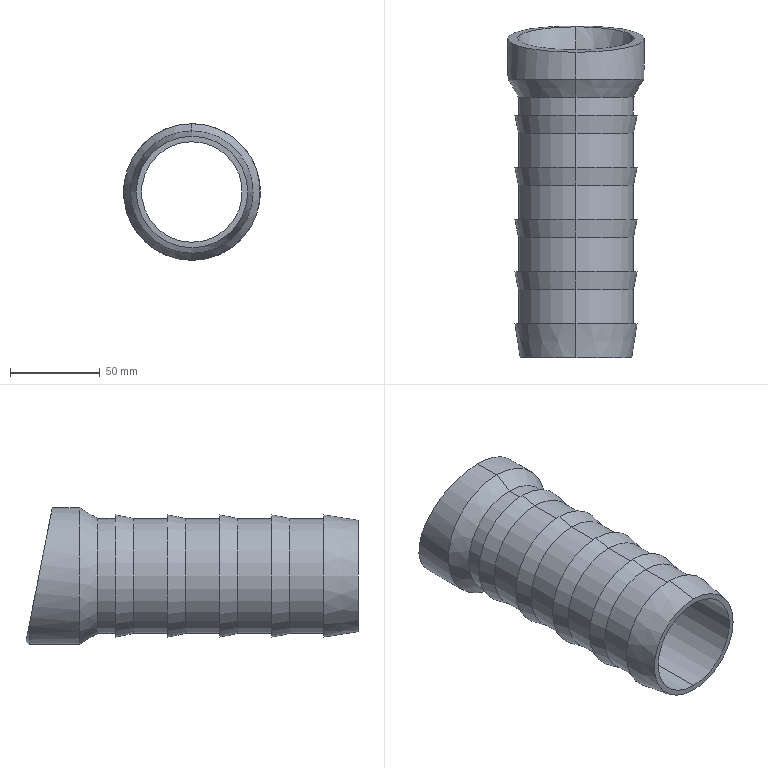Part | SolidWorks | features ICE 2, BlendCut 1, Revolution 1 | 1 solid | 37 faces | box 76 x 184.67 x 76 mm | volume 170240 mm3 | cone 16 | cylinder 14 | plane 7 | commonest cylinder face diameters 64 x10 56 x2 76 x2
STEP:
#1=CARTESIAN_POINT('',(0.,62.5,-28.));
#2=VERTEX_POINT('',#1);
#3=CARTESIAN_POINT('',(0.,62.5,28.));
#4=VERTEX_POINT('',#3);
#5=CARTESIAN_POINT('',(0.,62.5,0.));
#6=DIRECTION('',(0.,1.,0.));
#7=DIRECTION('',(0.,0.,1.));
#8=AXIS2_PLACEMENT_3D('',#5,#6,#7);
#9=CIRCLE('',#8,28.);
#10=EDGE_CURVE('',#2,#4,#9,.T.);
#11=ORIENTED_EDGE('',*,*,#10,.F.);
#12=CARTESIAN_POINT('',(0.,91.678,-33.836));
#13=VERTEX_POINT('',#12);
#14=CARTESIAN_POINT('',(0.,62.5,-28.));
#15=DIRECTION('',(0.,0.9806,-0.1961));
#16=VECTOR('',#15,1000.);
#17=LINE('',#14,#16);
#18=EDGE_CURVE('',#2,#13,#17,.T.);
#19=ORIENTED_EDGE('',*,*,#18,.T.);
#20=CARTESIAN_POINT('',(0.,78.829,31.266));
#21=VERTEX_POINT('',#20);
#22=CARTESIAN_POINT('',(0.,91.678,-33.836));
#23=CARTESIAN_POINT('',(-65.051,91.678,-33.836));
#24=CARTESIAN_POINT('',(-65.051,78.829,31.266));
#25=CARTESIAN_POINT('',(0.,78.829,31.266));
#26=(BOUNDED_CURVE()B_SPLINE_CURVE(3,(#22,#23,#24,#25),.UNSPECIFIED.,.F.,.F.)B_SPLINE_CURVE_WITH_KNOTS((4,4),(0.,3.142),.UNSPECIFIED.)CURVE()GEOMETRIC_REPRESENTATION_ITEM()RATIONAL_B_SPLINE_CURVE((1.,0.3333,0.3333,1.))REPRESENTATION_ITEM(''));
#27=EDGE_CURVE('',#13,#21,#26,.T.);
#28=ORIENTED_EDGE('',*,*,#27,.T.);
#29=CARTESIAN_POINT('',(0.,62.5,28.));
#30=DIRECTION('',(0.,0.9806,0.1961));
#31=VECTOR('',#30,1000.);
#32=LINE('',#29,#31);
#33=EDGE_CURVE('',#4,#21,#32,.T.);
#34=ORIENTED_EDGE('',*,*,#33,.F.);
#35=EDGE_LOOP('',(#11,#19,#28,#34));
#36=FACE_OUTER_BOUND('',#35,.T.);
#37=CARTESIAN_POINT('',(0.,62.5,0.));
#38=DIRECTION('',(0.,1.,0.));
#39=DIRECTION('',(0.,0.,1.));
#40=AXIS2_PLACEMENT_3D('',#37,#38,#39);
#41=CONICAL_SURFACE('',#40,28.,0.1974);
#42=ADVANCED_FACE('',(#36),#41,.F.);
#43=CARTESIAN_POINT('',(0.,-92.5,28.));
#44=VERTEX_POINT('',#43);
#45=CARTESIAN_POINT('',(0.,-92.5,-28.));
#46=VERTEX_POINT('',#45);
#47=CARTESIAN_POINT('',(0.,-92.5,0.));
#48=DIRECTION('',(0.,-1.,0.));
#49=DIRECTION('',(0.,0.,1.));
#50=AXIS2_PLACEMENT_3D('',#47,#48,#49);
#51=CIRCLE('',#50,28.);
#52=EDGE_CURVE('',#44,#46,#51,.T.);
#53=ORIENTED_EDGE('',*,*,#52,.T.);
#54=CARTESIAN_POINT('',(0.,-171.696,-28.));
#55=DIRECTION('',(0.,1.,0.));
#56=VECTOR('',#55,1000.);
#57=LINE('',#54,#56);
#58=EDGE_CURVE('',#46,#2,#57,.T.);
#59=ORIENTED_EDGE('',*,*,#58,.T.);
#60=ORIENTED_EDGE('',*,*,#10,.T.);
#61=CARTESIAN_POINT('',(0.,-171.696,28.));
#62=DIRECTION('',(0.,1.,0.));
#63=VECTOR('',#62,1000.);
#64=LINE('',#61,#63);
#65=EDGE_CURVE('',#44,#4,#64,.T.);
#66=ORIENTED_EDGE('',*,*,#65,.F.);
#67=EDGE_LOOP('',(#53,#59,#60,#66));
#68=FACE_OUTER_BOUND('',#67,.T.);
#69=CARTESIAN_POINT('',(0.,-171.696,0.));
#70=DIRECTION('',(0.,1.,0.));
#71=DIRECTION('',(0.,0.,1.));
#72=AXIS2_PLACEMENT_3D('',#69,#70,#71);
#73=CYLINDRICAL_SURFACE('',#72,28.);
#74=ADVANCED_FACE('',(#68),#73,.F.);
#75=CARTESIAN_POINT('',(0.,-54.5,32.));
#76=VERTEX_POINT('',#75);
#77=CARTESIAN_POINT('',(0.,-54.5,-32.));
#78=VERTEX_POINT('',#77);
#79=CARTESIAN_POINT('',(0.,-54.5,0.));
#80=DIRECTION('',(0.,1.,0.));
#81=DIRECTION('',(0.,0.,1.));
#82=AXIS2_PLACEMENT_3D('',#79,#80,#81);
#83=CIRCLE('',#82,32.);
#84=EDGE_CURVE('',#76,#78,#83,.T.);
#85=ORIENTED_EDGE('',*,*,#84,.T.);
#86=CARTESIAN_POINT('',(0.,-44.5,-34.));
#87=VERTEX_POINT('',#86);
#88=CARTESIAN_POINT('',(0.,-54.5,-32.));
#89=DIRECTION('',(0.,0.9806,-0.1961));
#90=VECTOR('',#89,1000.);
#91=LINE('',#88,#90);
#92=EDGE_CURVE('',#78,#87,#91,.T.);
#93=ORIENTED_EDGE('',*,*,#92,.T.);
#94=CARTESIAN_POINT('',(0.,-44.5,34.));
#95=VERTEX_POINT('',#94);
#96=CARTESIAN_POINT('',(0.,-44.5,0.));
#97=DIRECTION('',(0.,1.,0.));
#98=DIRECTION('',(0.,0.,1.));
#99=AXIS2_PLACEMENT_3D('',#96,#97,#98);
#100=CIRCLE('',#99,34.);
#101=EDGE_CURVE('',#95,#87,#100,.T.);
#102=ORIENTED_EDGE('',*,*,#101,.F.);
#103=CARTESIAN_POINT('',(0.,-54.5,32.));
#104=DIRECTION('',(0.,0.9806,0.1961));
#105=VECTOR('',#104,1000.);
#106=LINE('',#103,#105);
#107=EDGE_CURVE('',#76,#95,#106,.T.);
#108=ORIENTED_EDGE('',*,*,#107,.F.);
#109=EDGE_LOOP('',(#85,#93,#102,#108));
#110=FACE_OUTER_BOUND('',#109,.T.);
#111=CARTESIAN_POINT('',(0.,-54.5,0.));
#112=DIRECTION('',(0.,1.,0.));
#113=DIRECTION('',(0.,0.,1.));
#114=AXIS2_PLACEMENT_3D('',#111,#112,#113);
#115=CONICAL_SURFACE('',#114,32.,0.1974);
#116=ADVANCED_FACE('',(#110),#115,.T.);
#117=CARTESIAN_POINT('',(0.,-73.5,32.));
#118=VERTEX_POINT('',#117);
#119=CARTESIAN_POINT('',(0.,-73.5,-32.));
#120=VERTEX_POINT('',#119);
#121=CARTESIAN_POINT('',(0.,-73.5,0.));
#122=DIRECTION('',(0.,1.,0.));
#123=DIRECTION('',(0.,0.,1.));
#124=AXIS2_PLACEMENT_3D('',#121,#122,#123);
#125=CIRCLE('',#124,32.);
#126=EDGE_CURVE('',#118,#120,#125,.T.);
#127=ORIENTED_EDGE('',*,*,#126,.T.);
#128=CARTESIAN_POINT('',(0.,92.5,-32.));
#129=DIRECTION('',(0.,1.,0.));
#130=VECTOR('',#129,1000.);
#131=LINE('',#128,#130);
#132=EDGE_CURVE('',#120,#78,#131,.T.);
#133=ORIENTED_EDGE('',*,*,#132,.T.);
#134=ORIENTED_EDGE('',*,*,#84,.F.);
#135=CARTESIAN_POINT('',(0.,92.5,32.));
#136=DIRECTION('',(0.,1.,0.));
#137=VECTOR('',#136,1000.);
#138=LINE('',#135,#137);
#139=EDGE_CURVE('',#118,#76,#138,.T.);
#140=ORIENTED_EDGE('',*,*,#139,.F.);
#141=EDGE_LOOP('',(#127,#133,#134,#140));
#142=FACE_OUTER_BOUND('',#141,.T.);
#143=CARTESIAN_POINT('',(0.,92.5,0.));
#144=DIRECTION('',(0.,1.,0.));
#145=DIRECTION('',(0.,0.,1.));
#146=AXIS2_PLACEMENT_3D('',#143,#144,#145);
#147=CYLINDRICAL_SURFACE('',#146,32.);
#148=ADVANCED_FACE('',(#142),#147,.T.);
#149=CARTESIAN_POINT('',(0.,-92.5,31.));
#150=VERTEX_POINT('',#149);
#151=CARTESIAN_POINT('',(0.,-92.5,-31.));
#152=VERTEX_POINT('',#151);
#153=CARTESIAN_POINT('',(0.,-92.5,0.));
#154=DIRECTION('',(0.,1.,0.));
#155=DIRECTION('',(0.,0.,1.));
#156=AXIS2_PLACEMENT_3D('',#153,#154,#155);
#157=CIRCLE('',#156,31.);
#158=EDGE_CURVE('',#150,#152,#157,.T.);
#159=ORIENTED_EDGE('',*,*,#158,.T.);
#160=CARTESIAN_POINT('',(0.,-73.5,-34.));
#161=VERTEX_POINT('',#160);
#162=CARTESIAN_POINT('',(0.,-92.5,-31.));
#163=DIRECTION('',(0.,0.9878,-0.156));
#164=VECTOR('',#163,1000.);
#165=LINE('',#162,#164);
#166=EDGE_CURVE('',#152,#161,#165,.T.);
#167=ORIENTED_EDGE('',*,*,#166,.T.);
#168=CARTESIAN_POINT('',(0.,-73.5,34.));
#169=VERTEX_POINT('',#168);
#170=CARTESIAN_POINT('',(0.,-73.5,0.));
#171=DIRECTION('',(0.,1.,0.));
#172=DIRECTION('',(0.,0.,1.));
#173=AXIS2_PLACEMENT_3D('',#170,#171,#172);
#174=CIRCLE('',#173,34.);
#175=EDGE_CURVE('',#169,#161,#174,.T.);
#176=ORIENTED_EDGE('',*,*,#175,.F.);
#177=CARTESIAN_POINT('',(0.,-92.5,31.));
#178=DIRECTION('',(0.,0.9878,0.156));
#179=VECTOR('',#178,1000.);
#180=LINE('',#177,#179);
#181=EDGE_CURVE('',#150,#169,#180,.T.);
#182=ORIENTED_EDGE('',*,*,#181,.F.);
#183=EDGE_LOOP('',(#159,#167,#176,#182));
#184=FACE_OUTER_BOUND('',#183,.T.);
#185=CARTESIAN_POINT('',(0.,-92.5,0.));
#186=DIRECTION('',(0.,1.,0.));
#187=DIRECTION('',(0.,0.,1.));
#188=AXIS2_PLACEMENT_3D('',#185,#186,#187);
#189=CONICAL_SURFACE('',#188,31.,0.1566);
#190=ADVANCED_FACE('',(#184),#189,.T.);
#191=CARTESIAN_POINT('',(-25.835,90.5,-27.867));
#192=VERTEX_POINT('',#191);
#193=CARTESIAN_POINT('',(0.,92.17,-36.33));
#194=VERTEX_POINT('',#193);
#195=CARTESIAN_POINT('',(-25.835,90.5,-27.867));
#196=CARTESIAN_POINT('',(-18.239,91.595,-33.416));
#197=CARTESIAN_POINT('',(-9.343,92.17,-36.33));
#198=CARTESIAN_POINT('',(0.,92.17,-36.33));
#199=(BOUNDED_CURVE()B_SPLINE_CURVE(3,(#195,#196,#197,#198),.UNSPECIFIED.,.F.,.F.)B_SPLINE_CURVE_WITH_KNOTS((4,4),(2.52,3.142),.UNSPECIFIED.)CURVE()GEOMETRIC_REPRESENTATION_ITEM()RATIONAL_B_SPLINE_CURVE((1.,0.9681,0.9681,1.))REPRESENTATION_ITEM(''));
#200=EDGE_CURVE('',#192,#194,#199,.T.);
#201=ORIENTED_EDGE('',*,*,#200,.T.);
#202=CARTESIAN_POINT('',(0.,90.5,-38.));
#203=VERTEX_POINT('',#202);
#204=CARTESIAN_POINT('',(0.,90.5,-38.));
#205=DIRECTION('',(0.,-0.7071,-0.7071));
#206=VECTOR('',#205,1000.);
#207=LINE('',#204,#206);
#208=EDGE_CURVE('',#194,#203,#207,.T.);
#209=ORIENTED_EDGE('',*,*,#208,.T.);
#210=CARTESIAN_POINT('',(0.,90.5,0.));
#211=DIRECTION('',(0.,1.,0.));
#212=DIRECTION('',(0.,0.,1.));
#213=AXIS2_PLACEMENT_3D('',#210,#211,#212);
#214=CIRCLE('',#213,38.);
#215=EDGE_CURVE('',#203,#192,#214,.T.);
#216=ORIENTED_EDGE('',*,*,#215,.T.);
#217=EDGE_LOOP('',(#201,#209,#216));
#218=FACE_OUTER_BOUND('',#217,.T.);
#219=CARTESIAN_POINT('',(0.,90.5,0.));
#220=DIRECTION('',(0.,-1.,0.));
#221=DIRECTION('',(0.,0.,-1.));
#222=AXIS2_PLACEMENT_3D('',#219,#220,#221);
#223=CONICAL_SURFACE('',#222,38.,0.7854);
#224=ADVANCED_FACE('',(#218),#223,.T.);
#225=CARTESIAN_POINT('',(0.,62.5,38.));
#226=VERTEX_POINT('',#225);
#227=CARTESIAN_POINT('',(0.,62.5,-38.));
#228=VERTEX_POINT('',#227);
#229=CARTESIAN_POINT('',(0.,62.5,0.));
#230=DIRECTION('',(0.,1.,0.));
#231=DIRECTION('',(0.,0.,1.));
#232=AXIS2_PLACEMENT_3D('',#229,#230,#231);
#233=CIRCLE('',#232,38.);
#234=EDGE_CURVE('',#226,#228,#233,.T.);
#235=ORIENTED_EDGE('',*,*,#234,.T.);
#236=CARTESIAN_POINT('',(0.,92.5,-38.));
#237=DIRECTION('',(0.,1.,0.));
#238=VECTOR('',#237,1000.);
#239=LINE('',#236,#238);
#240=EDGE_CURVE('',#228,#203,#239,.T.);
#241=ORIENTED_EDGE('',*,*,#240,.T.);
#242=CARTESIAN_POINT('',(25.835,90.5,-27.867));
#243=VERTEX_POINT('',#242);
#244=CARTESIAN_POINT('',(0.,90.5,0.));
#245=DIRECTION('',(0.,1.,0.));
#246=DIRECTION('',(0.,0.,1.));
#247=AXIS2_PLACEMENT_3D('',#244,#245,#246);
#248=CIRCLE('',#247,38.);
#249=EDGE_CURVE('',#243,#203,#248,.T.);
#250=ORIENTED_EDGE('',*,*,#249,.F.);
#251=CARTESIAN_POINT('',(0.,77.5,38.));
#252=VERTEX_POINT('',#251);
#253=CARTESIAN_POINT('',(25.835,90.5,-27.867));
#254=CARTESIAN_POINT('',(55.821,85.013,-0.06669));
#255=CARTESIAN_POINT('',(40.89,77.5,38.));
#256=CARTESIAN_POINT('',(0.,77.5,38.));
#257=(BOUNDED_CURVE()B_SPLINE_CURVE(3,(#253,#254,#255,#256),.UNSPECIFIED.,.F.,.F.)B_SPLINE_CURVE_WITH_KNOTS((4,4),(0.7476,3.142),.UNSPECIFIED.)CURVE()GEOMETRIC_REPRESENTATION_ITEM()RATIONAL_B_SPLINE_CURVE((1.,0.5768,0.5768,1.))REPRESENTATION_ITEM(''));
#258=EDGE_CURVE('',#243,#252,#257,.T.);
#259=ORIENTED_EDGE('',*,*,#258,.T.);
#260=CARTESIAN_POINT('',(0.,92.5,38.));
#261=DIRECTION('',(0.,1.,0.));
#262=VECTOR('',#261,1000.);
#263=LINE('',#260,#262);
#264=EDGE_CURVE('',#226,#252,#263,.T.);
#265=ORIENTED_EDGE('',*,*,#264,.F.);
#266=EDGE_LOOP('',(#235,#241,#250,#259,#265));
#267=FACE_OUTER_BOUND('',#266,.T.);
#268=CARTESIAN_POINT('',(0.,92.5,0.));
#269=DIRECTION('',(0.,1.,0.));
#270=DIRECTION('',(0.,0.,1.));
#271=AXIS2_PLACEMENT_3D('',#268,#269,#270);
#272=CYLINDRICAL_SURFACE('',#271,38.);
#273=ADVANCED_FACE('',(#267),#272,.T.);
#274=CARTESIAN_POINT('',(0.,52.5,32.));
#275=VERTEX_POINT('',#274);
#276=CARTESIAN_POINT('',(0.,52.5,-32.));
#277=VERTEX_POINT('',#276);
#278=CARTESIAN_POINT('',(0.,52.5,0.));
#279=DIRECTION('',(0.,1.,0.));
#280=DIRECTION('',(0.,0.,1.));
#281=AXIS2_PLACEMENT_3D('',#278,#279,#280);
#282=CIRCLE('',#281,32.);
#283=EDGE_CURVE('',#275,#277,#282,.T.);
#284=ORIENTED_EDGE('',*,*,#283,.T.);
#285=CARTESIAN_POINT('',(0.,52.5,-32.));
#286=DIRECTION('',(0.,0.8575,-0.5145));
#287=VECTOR('',#286,1000.);
#288=LINE('',#285,#287);
#289=EDGE_CURVE('',#277,#228,#288,.T.);
#290=ORIENTED_EDGE('',*,*,#289,.T.);
#291=ORIENTED_EDGE('',*,*,#234,.F.);
#292=CARTESIAN_POINT('',(0.,52.5,32.));
#293=DIRECTION('',(0.,0.8575,0.5145));
#294=VECTOR('',#293,1000.);
#295=LINE('',#292,#294);
#296=EDGE_CURVE('',#275,#226,#295,.T.);
#297=ORIENTED_EDGE('',*,*,#296,.F.);
#298=EDGE_LOOP('',(#284,#290,#291,#297));
#299=FACE_OUTER_BOUND('',#298,.T.);
#300=CARTESIAN_POINT('',(0.,52.5,0.));
#301=DIRECTION('',(0.,1.,0.));
#302=DIRECTION('',(0.,0.,1.));
#303=AXIS2_PLACEMENT_3D('',#300,#301,#302);
#304=CONICAL_SURFACE('',#303,32.,0.5404);
#305=ADVANCED_FACE('',(#299),#304,.T.);
#306=CARTESIAN_POINT('',(0.,42.5,32.));
#307=VERTEX_POINT('',#306);
#308=CARTESIAN_POINT('',(0.,42.5,-32.));
#309=VERTEX_POINT('',#308);
#310=CARTESIAN_POINT('',(0.,42.5,0.));
#311=DIRECTION('',(0.,1.,0.));
#312=DIRECTION('',(0.,0.,1.));
#313=AXIS2_PLACEMENT_3D('',#310,#311,#312);
#314=CIRCLE('',#313,32.);
#315=EDGE_CURVE('',#307,#309,#314,.T.);
#316=ORIENTED_EDGE('',*,*,#315,.T.);
#317=CARTESIAN_POINT('',(0.,92.5,-32.));
#318=DIRECTION('',(0.,1.,0.));
#319=VECTOR('',#318,1000.);
#320=LINE('',#317,#319);
#321=EDGE_CURVE('',#309,#277,#320,.T.);
#322=ORIENTED_EDGE('',*,*,#321,.T.);
#323=ORIENTED_EDGE('',*,*,#283,.F.);
#324=CARTESIAN_POINT('',(0.,92.5,32.));
#325=DIRECTION('',(0.,1.,0.));
#326=VECTOR('',#325,1000.);
#327=LINE('',#324,#326);
#328=EDGE_CURVE('',#307,#275,#327,.T.);
#329=ORIENTED_EDGE('',*,*,#328,.F.);
#330=EDGE_LOOP('',(#316,#322,#323,#329));
#331=FACE_OUTER_BOUND('',#330,.T.);
#332=CARTESIAN_POINT('',(0.,92.5,0.));
#333=DIRECTION('',(0.,1.,0.));
#334=DIRECTION('',(0.,0.,1.));
#335=AXIS2_PLACEMENT_3D('',#332,#333,#334);
#336=CYLINDRICAL_SURFACE('',#335,32.);
#337=ADVANCED_FACE('',(#331),#336,.T.);
#338=CARTESIAN_POINT('',(0.,32.5,32.));
#339=VERTEX_POINT('',#338);
#340=CARTESIAN_POINT('',(0.,32.5,-32.));
#341=VERTEX_POINT('',#340);
#342=CARTESIAN_POINT('',(0.,32.5,0.));
#343=DIRECTION('',(0.,1.,0.));
#344=DIRECTION('',(0.,0.,1.));
#345=AXIS2_PLACEMENT_3D('',#342,#343,#344);
#346=CIRCLE('',#345,32.);
#347=EDGE_CURVE('',#339,#341,#346,.T.);
#348=ORIENTED_EDGE('',*,*,#347,.T.);
#349=CARTESIAN_POINT('',(0.,42.5,-34.));
#350=VERTEX_POINT('',#349);
#351=CARTESIAN_POINT('',(0.,32.5,-32.));
#352=DIRECTION('',(0.,0.9806,-0.1961));
#353=VECTOR('',#352,1000.);
#354=LINE('',#351,#353);
#355=EDGE_CURVE('',#341,#350,#354,.T.);
#356=ORIENTED_EDGE('',*,*,#355,.T.);
#357=CARTESIAN_POINT('',(0.,42.5,34.));
#358=VERTEX_POINT('',#357);
#359=CARTESIAN_POINT('',(0.,42.5,0.));
#360=DIRECTION('',(0.,1.,0.));
#361=DIRECTION('',(0.,0.,1.));
#362=AXIS2_PLACEMENT_3D('',#359,#360,#361);
#363=CIRCLE('',#362,34.);
#364=EDGE_CURVE('',#358,#350,#363,.T.);
#365=ORIENTED_EDGE('',*,*,#364,.F.);
#366=CARTESIAN_POINT('',(0.,32.5,32.));
#367=DIRECTION('',(0.,0.9806,0.1961));
#368=VECTOR('',#367,1000.);
#369=LINE('',#366,#368);
#370=EDGE_CURVE('',#339,#358,#369,.T.);
#371=ORIENTED_EDGE('',*,*,#370,.F.);
#372=EDGE_LOOP('',(#348,#356,#365,#371));
#373=FACE_OUTER_BOUND('',#372,.T.);
#374=CARTESIAN_POINT('',(0.,32.5,0.));
#375=DIRECTION('',(0.,1.,0.));
#376=DIRECTION('',(0.,0.,1.));
#377=AXIS2_PLACEMENT_3D('',#374,#375,#376);
#378=CONICAL_SURFACE('',#377,32.,0.1974);
#379=ADVANCED_FACE('',(#373),#378,.T.);
#380=CARTESIAN_POINT('',(0.,13.5,32.));
#381=VERTEX_POINT('',#380);
#382=CARTESIAN_POINT('',(0.,13.5,-32.));
#383=VERTEX_POINT('',#382);
#384=CARTESIAN_POINT('',(0.,13.5,0.));
#385=DIRECTION('',(0.,1.,0.));
#386=DIRECTION('',(0.,0.,1.));
#387=AXIS2_PLACEMENT_3D('',#384,#385,#386);
#388=CIRCLE('',#387,32.);
#389=EDGE_CURVE('',#381,#383,#388,.T.);
#390=ORIENTED_EDGE('',*,*,#389,.T.);
#391=CARTESIAN_POINT('',(0.,92.5,-32.));
#392=DIRECTION('',(0.,1.,0.));
#393=VECTOR('',#392,1000.);
#394=LINE('',#391,#393);
#395=EDGE_CURVE('',#383,#341,#394,.T.);
#396=ORIENTED_EDGE('',*,*,#395,.T.);
#397=ORIENTED_EDGE('',*,*,#347,.F.);
#398=CARTESIAN_POINT('',(0.,92.5,32.));
#399=DIRECTION('',(0.,1.,0.));
#400=VECTOR('',#399,1000.);
#401=LINE('',#398,#400);
#402=EDGE_CURVE('',#381,#339,#401,.T.);
#403=ORIENTED_EDGE('',*,*,#402,.F.);
#404=EDGE_LOOP('',(#390,#396,#397,#403));
#405=FACE_OUTER_BOUND('',#404,.T.);
#406=CARTESIAN_POINT('',(0.,92.5,0.));
#407=DIRECTION('',(0.,1.,0.));
#408=DIRECTION('',(0.,0.,1.));
#409=AXIS2_PLACEMENT_3D('',#406,#407,#408);
#410=CYLINDRICAL_SURFACE('',#409,32.);
#411=ADVANCED_FACE('',(#405),#410,.T.);
#412=CARTESIAN_POINT('',(0.,3.5,32.));
#413=VERTEX_POINT('',#412);
#414=CARTESIAN_POINT('',(0.,3.5,-32.));
#415=VERTEX_POINT('',#414);
#416=CARTESIAN_POINT('',(0.,3.5,0.));
#417=DIRECTION('',(0.,1.,0.));
#418=DIRECTION('',(0.,0.,1.));
#419=AXIS2_PLACEMENT_3D('',#416,#417,#418);
#420=CIRCLE('',#419,32.);
#421=EDGE_CURVE('',#413,#415,#420,.T.);
#422=ORIENTED_EDGE('',*,*,#421,.T.);
#423=CARTESIAN_POINT('',(0.,13.5,-34.));
#424=VERTEX_POINT('',#423);
#425=CARTESIAN_POINT('',(0.,3.5,-32.));
#426=DIRECTION('',(0.,0.9806,-0.1961));
#427=VECTOR('',#426,1000.);
#428=LINE('',#425,#427);
#429=EDGE_CURVE('',#415,#424,#428,.T.);
#430=ORIENTED_EDGE('',*,*,#429,.T.);
#431=CARTESIAN_POINT('',(0.,13.5,34.));
#432=VERTEX_POINT('',#431);
#433=CARTESIAN_POINT('',(0.,13.5,0.));
#434=DIRECTION('',(0.,1.,0.));
#435=DIRECTION('',(0.,0.,1.));
#436=AXIS2_PLACEMENT_3D('',#433,#434,#435);
#437=CIRCLE('',#436,34.);
#438=EDGE_CURVE('',#432,#424,#437,.T.);
#439=ORIENTED_EDGE('',*,*,#438,.F.);
#440=CARTESIAN_POINT('',(0.,3.5,32.));
#441=DIRECTION('',(0.,0.9806,0.1961));
#442=VECTOR('',#441,1000.);
#443=LINE('',#440,#442);
#444=EDGE_CURVE('',#413,#432,#443,.T.);
#445=ORIENTED_EDGE('',*,*,#444,.F.);
#446=EDGE_LOOP('',(#422,#430,#439,#445));
#447=FACE_OUTER_BOUND('',#446,.T.);
#448=CARTESIAN_POINT('',(0.,3.5,0.));
#449=DIRECTION('',(0.,1.,0.));
#450=DIRECTION('',(0.,0.,1.));
#451=AXIS2_PLACEMENT_3D('',#448,#449,#450);
#452=CONICAL_SURFACE('',#451,32.,0.1974);
#453=ADVANCED_FACE('',(#447),#452,.T.);
#454=CARTESIAN_POINT('',(0.,-15.5,32.));
#455=VERTEX_POINT('',#454);
#456=CARTESIAN_POINT('',(0.,-15.5,-32.));
#457=VERTEX_POINT('',#456);
#458=CARTESIAN_POINT('',(0.,-15.5,0.));
#459=DIRECTION('',(0.,1.,0.));
#460=DIRECTION('',(0.,0.,1.));
#461=AXIS2_PLACEMENT_3D('',#458,#459,#460);
#462=CIRCLE('',#461,32.);
#463=EDGE_CURVE('',#455,#457,#462,.T.);
#464=ORIENTED_EDGE('',*,*,#463,.T.);
#465=CARTESIAN_POINT('',(0.,92.5,-32.));
#466=DIRECTION('',(0.,1.,0.));
#467=VECTOR('',#466,1000.);
#468=LINE('',#465,#467);
#469=EDGE_CURVE('',#457,#415,#468,.T.);
#470=ORIENTED_EDGE('',*,*,#469,.T.);
#471=ORIENTED_EDGE('',*,*,#421,.F.);
#472=CARTESIAN_POINT('',(0.,92.5,32.));
#473=DIRECTION('',(0.,1.,0.));
#474=VECTOR('',#473,1000.);
#475=LINE('',#472,#474);
#476=EDGE_CURVE('',#455,#413,#475,.T.);
#477=ORIENTED_EDGE('',*,*,#476,.F.);
#478=EDGE_LOOP('',(#464,#470,#471,#477));
#479=FACE_OUTER_BOUND('',#478,.T.);
#480=CARTESIAN_POINT('',(0.,92.5,0.));
#481=DIRECTION('',(0.,1.,0.));
#482=DIRECTION('',(0.,0.,1.));
#483=AXIS2_PLACEMENT_3D('',#480,#481,#482);
#484=CYLINDRICAL_SURFACE('',#483,32.);
#485=ADVANCED_FACE('',(#479),#484,.T.);
#486=CARTESIAN_POINT('',(0.,-25.5,32.));
#487=VERTEX_POINT('',#486);
#488=CARTESIAN_POINT('',(0.,-25.5,-32.));
#489=VERTEX_POINT('',#488);
#490=CARTESIAN_POINT('',(0.,-25.5,0.));
#491=DIRECTION('',(0.,1.,0.));
#492=DIRECTION('',(0.,0.,1.));
#493=AXIS2_PLACEMENT_3D('',#490,#491,#492);
#494=CIRCLE('',#493,32.);
#495=EDGE_CURVE('',#487,#489,#494,.T.);
#496=ORIENTED_EDGE('',*,*,#495,.T.);
#497=CARTESIAN_POINT('',(0.,-15.5,-34.));
#498=VERTEX_POINT('',#497);
#499=CARTESIAN_POINT('',(0.,-25.5,-32.));
#500=DIRECTION('',(0.,0.9806,-0.1961));
#501=VECTOR('',#500,1000.);
#502=LINE('',#499,#501);
#503=EDGE_CURVE('',#489,#498,#502,.T.);
#504=ORIENTED_EDGE('',*,*,#503,.T.);
#505=CARTESIAN_POINT('',(0.,-15.5,34.));
#506=VERTEX_POINT('',#505);
#507=CARTESIAN_POINT('',(0.,-15.5,0.));
#508=DIRECTION('',(0.,1.,0.));
#509=DIRECTION('',(0.,0.,1.));
#510=AXIS2_PLACEMENT_3D('',#507,#508,#509);
#511=CIRCLE('',#510,34.);
#512=EDGE_CURVE('',#506,#498,#511,.T.);
#513=ORIENTED_EDGE('',*,*,#512,.F.);
#514=CARTESIAN_POINT('',(0.,-25.5,32.));
#515=DIRECTION('',(0.,0.9806,0.1961));
#516=VECTOR('',#515,1000.);
#517=LINE('',#514,#516);
#518=EDGE_CURVE('',#487,#506,#517,.T.);
#519=ORIENTED_EDGE('',*,*,#518,.F.);
#520=EDGE_LOOP('',(#496,#504,#513,#519));
#521=FACE_OUTER_BOUND('',#520,.T.);
#522=CARTESIAN_POINT('',(0.,-25.5,0.));
#523=DIRECTION('',(0.,1.,0.));
#524=DIRECTION('',(0.,0.,1.));
#525=AXIS2_PLACEMENT_3D('',#522,#523,#524);
#526=CONICAL_SURFACE('',#525,32.,0.1974);
#527=ADVANCED_FACE('',(#521),#526,.T.);
#528=CARTESIAN_POINT('',(0.,-44.5,32.));
#529=VERTEX_POINT('',#528);
#530=CARTESIAN_POINT('',(0.,-44.5,-32.));
#531=VERTEX_POINT('',#530);
#532=CARTESIAN_POINT('',(0.,-44.5,0.));
#533=DIRECTION('',(0.,1.,0.));
#534=DIRECTION('',(0.,0.,1.));
#535=AXIS2_PLACEMENT_3D('',#532,#533,#534);
#536=CIRCLE('',#535,32.);
#537=EDGE_CURVE('',#529,#531,#536,.T.);
#538=ORIENTED_EDGE('',*,*,#537,.T.);
#539=CARTESIAN_POINT('',(0.,92.5,-32.));
#540=DIRECTION('',(0.,1.,0.));
#541=VECTOR('',#540,1000.);
#542=LINE('',#539,#541);
#543=EDGE_CURVE('',#531,#489,#542,.T.);
#544=ORIENTED_EDGE('',*,*,#543,.T.);
#545=ORIENTED_EDGE('',*,*,#495,.F.);
#546=CARTESIAN_POINT('',(0.,92.5,32.));
#547=DIRECTION('',(0.,1.,0.));
#548=VECTOR('',#547,1000.);
#549=LINE('',#546,#548);
#550=EDGE_CURVE('',#529,#487,#549,.T.);
#551=ORIENTED_EDGE('',*,*,#550,.F.);
#552=EDGE_LOOP('',(#538,#544,#545,#551));
#553=FACE_OUTER_BOUND('',#552,.T.);
#554=CARTESIAN_POINT('',(0.,92.5,0.));
#555=DIRECTION('',(0.,1.,0.));
#556=DIRECTION('',(0.,0.,1.));
#557=AXIS2_PLACEMENT_3D('',#554,#555,#556);
#558=CYLINDRICAL_SURFACE('',#557,32.);
#559=ADVANCED_FACE('',(#553),#558,.T.);
#560=ORIENTED_EDGE('',*,*,#543,.F.);
#561=CARTESIAN_POINT('',(0.,-44.5,0.));
#562=DIRECTION('',(0.,1.,0.));
#563=DIRECTION('',(0.,0.,1.));
#564=AXIS2_PLACEMENT_3D('',#561,#562,#563);
#565=CIRCLE('',#564,32.);
#566=EDGE_CURVE('',#531,#529,#565,.T.);
#567=ORIENTED_EDGE('',*,*,#566,.T.);
#568=ORIENTED_EDGE('',*,*,#550,.T.);
#569=CARTESIAN_POINT('',(0.,-25.5,0.));
#570=DIRECTION('',(0.,1.,0.));
#571=DIRECTION('',(0.,0.,1.));
#572=AXIS2_PLACEMENT_3D('',#569,#570,#571);
#573=CIRCLE('',#572,32.);
#574=EDGE_CURVE('',#489,#487,#573,.T.);
#575=ORIENTED_EDGE('',*,*,#574,.F.);
#576=EDGE_LOOP('',(#560,#567,#568,#575));
#577=FACE_OUTER_BOUND('',#576,.T.);
#578=CARTESIAN_POINT('',(0.,92.5,0.));
#579=DIRECTION('',(0.,1.,0.));
#580=DIRECTION('',(0.,0.,1.));
#581=AXIS2_PLACEMENT_3D('',#578,#579,#580);
#582=CYLINDRICAL_SURFACE('',#581,32.);
#583=ADVANCED_FACE('',(#577),#582,.T.);
#584=ORIENTED_EDGE('',*,*,#503,.F.);
#585=ORIENTED_EDGE('',*,*,#574,.T.);
#586=ORIENTED_EDGE('',*,*,#518,.T.);
#587=CARTESIAN_POINT('',(0.,-15.5,0.));
#588=DIRECTION('',(0.,1.,0.));
#589=DIRECTION('',(0.,0.,1.));
#590=AXIS2_PLACEMENT_3D('',#587,#588,#589);
#591=CIRCLE('',#590,34.);
#592=EDGE_CURVE('',#498,#506,#591,.T.);
#593=ORIENTED_EDGE('',*,*,#592,.F.);
#594=EDGE_LOOP('',(#584,#585,#586,#593));
#595=FACE_OUTER_BOUND('',#594,.T.);
#596=CARTESIAN_POINT('',(0.,-25.5,0.));
#597=DIRECTION('',(0.,1.,0.));
#598=DIRECTION('',(0.,0.,1.));
#599=AXIS2_PLACEMENT_3D('',#596,#597,#598);
#600=CONICAL_SURFACE('',#599,32.,0.1974);
#601=ADVANCED_FACE('',(#595),#600,.T.);
#602=ORIENTED_EDGE('',*,*,#463,.F.);
#603=CARTESIAN_POINT('',(0.,-15.5,0.));
#604=DIRECTION('',(0.,1.,0.));
#605=DIRECTION('',(0.,0.,1.));
#606=AXIS2_PLACEMENT_3D('',#603,#604,#605);
#607=CIRCLE('',#606,32.);
#608=EDGE_CURVE('',#457,#455,#607,.T.);
#609=ORIENTED_EDGE('',*,*,#608,.F.);
#610=EDGE_LOOP('',(#602,#609));
#611=FACE_BOUND('',#610,.T.);
#612=ORIENTED_EDGE('',*,*,#512,.T.);
#613=ORIENTED_EDGE('',*,*,#592,.T.);
#614=EDGE_LOOP('',(#612,#613));
#615=FACE_OUTER_BOUND('',#614,.T.);
#616=CARTESIAN_POINT('',(34.,-15.5,0.));
#617=DIRECTION('',(0.,-1.,0.));
#618=DIRECTION('',(0.,0.,-1.));
#619=AXIS2_PLACEMENT_3D('',#616,#617,#618);
#620=PLANE('',#619);
#621=ADVANCED_FACE('',(#611,#615),#620,.F.);
#622=ORIENTED_EDGE('',*,*,#469,.F.);
#623=ORIENTED_EDGE('',*,*,#608,.T.);
#624=ORIENTED_EDGE('',*,*,#476,.T.);
#625=CARTESIAN_POINT('',(0.,3.5,0.));
#626=DIRECTION('',(0.,1.,0.));
#627=DIRECTION('',(0.,0.,1.));
#628=AXIS2_PLACEMENT_3D('',#625,#626,#627);
#629=CIRCLE('',#628,32.);
#630=EDGE_CURVE('',#415,#413,#629,.T.);
#631=ORIENTED_EDGE('',*,*,#630,.F.);
#632=EDGE_LOOP('',(#622,#623,#624,#631));
#633=FACE_OUTER_BOUND('',#632,.T.);
#634=CARTESIAN_POINT('',(0.,92.5,0.));
#635=DIRECTION('',(0.,1.,0.));
#636=DIRECTION('',(0.,0.,1.));
#637=AXIS2_PLACEMENT_3D('',#634,#635,#636);
#638=CYLINDRICAL_SURFACE('',#637,32.);
#639=ADVANCED_FACE('',(#633),#638,.T.);
#640=ORIENTED_EDGE('',*,*,#429,.F.);
#641=ORIENTED_EDGE('',*,*,#630,.T.);
#642=ORIENTED_EDGE('',*,*,#444,.T.);
#643=CARTESIAN_POINT('',(0.,13.5,0.));
#644=DIRECTION('',(0.,1.,0.));
#645=DIRECTION('',(0.,0.,1.));
#646=AXIS2_PLACEMENT_3D('',#643,#644,#645);
#647=CIRCLE('',#646,34.);
#648=EDGE_CURVE('',#424,#432,#647,.T.);
#649=ORIENTED_EDGE('',*,*,#648,.F.);
#650=EDGE_LOOP('',(#640,#641,#642,#649));
#651=FACE_OUTER_BOUND('',#650,.T.);
#652=CARTESIAN_POINT('',(0.,3.5,0.));
#653=DIRECTION('',(0.,1.,0.));
#654=DIRECTION('',(0.,0.,1.));
#655=AXIS2_PLACEMENT_3D('',#652,#653,#654);
#656=CONICAL_SURFACE('',#655,32.,0.1974);
#657=ADVANCED_FACE('',(#651),#656,.T.);
#658=ORIENTED_EDGE('',*,*,#389,.F.);
#659=CARTESIAN_POINT('',(0.,13.5,0.));
#660=DIRECTION('',(0.,1.,0.));
#661=DIRECTION('',(0.,0.,1.));
#662=AXIS2_PLACEMENT_3D('',#659,#660,#661);
#663=CIRCLE('',#662,32.);
#664=EDGE_CURVE('',#383,#381,#663,.T.);
#665=ORIENTED_EDGE('',*,*,#664,.F.);
#666=EDGE_LOOP('',(#658,#665));
#667=FACE_BOUND('',#666,.T.);
#668=ORIENTED_EDGE('',*,*,#438,.T.);
#669=ORIENTED_EDGE('',*,*,#648,.T.);
#670=EDGE_LOOP('',(#668,#669));
#671=FACE_OUTER_BOUND('',#670,.T.);
#672=CARTESIAN_POINT('',(34.,13.5,0.));
#673=DIRECTION('',(0.,-1.,0.));
#674=DIRECTION('',(0.,0.,-1.));
#675=AXIS2_PLACEMENT_3D('',#672,#673,#674);
#676=PLANE('',#675);
#677=ADVANCED_FACE('',(#667,#671),#676,.F.);
#678=ORIENTED_EDGE('',*,*,#395,.F.);
#679=ORIENTED_EDGE('',*,*,#664,.T.);
#680=ORIENTED_EDGE('',*,*,#402,.T.);
#681=CARTESIAN_POINT('',(0.,32.5,0.));
#682=DIRECTION('',(0.,1.,0.));
#683=DIRECTION('',(0.,0.,1.));
#684=AXIS2_PLACEMENT_3D('',#681,#682,#683);
#685=CIRCLE('',#684,32.);
#686=EDGE_CURVE('',#341,#339,#685,.T.);
#687=ORIENTED_EDGE('',*,*,#686,.F.);
#688=EDGE_LOOP('',(#678,#679,#680,#687));
#689=FACE_OUTER_BOUND('',#688,.T.);
#690=CARTESIAN_POINT('',(0.,92.5,0.));
#691=DIRECTION('',(0.,1.,0.));
#692=DIRECTION('',(0.,0.,1.));
#693=AXIS2_PLACEMENT_3D('',#690,#691,#692);
#694=CYLINDRICAL_SURFACE('',#693,32.);
#695=ADVANCED_FACE('',(#689),#694,.T.);
#696=ORIENTED_EDGE('',*,*,#355,.F.);
#697=ORIENTED_EDGE('',*,*,#686,.T.);
#698=ORIENTED_EDGE('',*,*,#370,.T.);
#699=CARTESIAN_POINT('',(0.,42.5,0.));
#700=DIRECTION('',(0.,1.,0.));
#701=DIRECTION('',(0.,0.,1.));
#702=AXIS2_PLACEMENT_3D('',#699,#700,#701);
#703=CIRCLE('',#702,34.);
#704=EDGE_CURVE('',#350,#358,#703,.T.);
#705=ORIENTED_EDGE('',*,*,#704,.F.);
#706=EDGE_LOOP('',(#696,#697,#698,#705));
#707=FACE_OUTER_BOUND('',#706,.T.);
#708=CARTESIAN_POINT('',(0.,32.5,0.));
#709=DIRECTION('',(0.,1.,0.));
#710=DIRECTION('',(0.,0.,1.));
#711=AXIS2_PLACEMENT_3D('',#708,#709,#710);
#712=CONICAL_SURFACE('',#711,32.,0.1974);
#713=ADVANCED_FACE('',(#707),#712,.T.);
#714=ORIENTED_EDGE('',*,*,#315,.F.);
#715=CARTESIAN_POINT('',(0.,42.5,0.));
#716=DIRECTION('',(0.,1.,0.));
#717=DIRECTION('',(0.,0.,1.));
#718=AXIS2_PLACEMENT_3D('',#715,#716,#717);
#719=CIRCLE('',#718,32.);
#720=EDGE_CURVE('',#309,#307,#719,.T.);
#721=ORIENTED_EDGE('',*,*,#720,.F.);
#722=EDGE_LOOP('',(#714,#721));
#723=FACE_BOUND('',#722,.T.);
#724=ORIENTED_EDGE('',*,*,#364,.T.);
#725=ORIENTED_EDGE('',*,*,#704,.T.);
#726=EDGE_LOOP('',(#724,#725));
#727=FACE_OUTER_BOUND('',#726,.T.);
#728=CARTESIAN_POINT('',(34.,42.5,0.));
#729=DIRECTION('',(0.,-1.,0.));
#730=DIRECTION('',(0.,0.,-1.));
#731=AXIS2_PLACEMENT_3D('',#728,#729,#730);
#732=PLANE('',#731);
#733=ADVANCED_FACE('',(#723,#727),#732,.F.);
#734=ORIENTED_EDGE('',*,*,#321,.F.);
#735=ORIENTED_EDGE('',*,*,#720,.T.);
#736=ORIENTED_EDGE('',*,*,#328,.T.);
#737=CARTESIAN_POINT('',(0.,52.5,0.));
#738=DIRECTION('',(0.,1.,0.));
#739=DIRECTION('',(0.,0.,1.));
#740=AXIS2_PLACEMENT_3D('',#737,#738,#739);
#741=CIRCLE('',#740,32.);
#742=EDGE_CURVE('',#277,#275,#741,.T.);
#743=ORIENTED_EDGE('',*,*,#742,.F.);
#744=EDGE_LOOP('',(#734,#735,#736,#743));
#745=FACE_OUTER_BOUND('',#744,.T.);
#746=CARTESIAN_POINT('',(0.,92.5,0.));
#747=DIRECTION('',(0.,1.,0.));
#748=DIRECTION('',(0.,0.,1.));
#749=AXIS2_PLACEMENT_3D('',#746,#747,#748);
#750=CYLINDRICAL_SURFACE('',#749,32.);
#751=ADVANCED_FACE('',(#745),#750,.T.);
#752=ORIENTED_EDGE('',*,*,#289,.F.);
#753=ORIENTED_EDGE('',*,*,#742,.T.);
#754=ORIENTED_EDGE('',*,*,#296,.T.);
#755=CARTESIAN_POINT('',(0.,62.5,0.));
#756=DIRECTION('',(0.,1.,0.));
#757=DIRECTION('',(0.,0.,1.));
#758=AXIS2_PLACEMENT_3D('',#755,#756,#757);
#759=CIRCLE('',#758,38.);
#760=EDGE_CURVE('',#228,#226,#759,.T.);
#761=ORIENTED_EDGE('',*,*,#760,.F.);
#762=EDGE_LOOP('',(#752,#753,#754,#761));
#763=FACE_OUTER_BOUND('',#762,.T.);
#764=CARTESIAN_POINT('',(0.,52.5,0.));
#765=DIRECTION('',(0.,1.,0.));
#766=DIRECTION('',(0.,0.,1.));
#767=AXIS2_PLACEMENT_3D('',#764,#765,#766);
#768=CONICAL_SURFACE('',#767,32.,0.5404);
#769=ADVANCED_FACE('',(#763),#768,.T.);
#770=ORIENTED_EDGE('',*,*,#240,.F.);
#771=ORIENTED_EDGE('',*,*,#760,.T.);
#772=ORIENTED_EDGE('',*,*,#264,.T.);
#773=CARTESIAN_POINT('',(0.,77.5,38.));
#774=CARTESIAN_POINT('',(-40.89,77.5,38.));
#775=CARTESIAN_POINT('',(-55.821,85.013,-0.06669));
#776=CARTESIAN_POINT('',(-25.835,90.5,-27.867));
#777=(BOUNDED_CURVE()B_SPLINE_CURVE(3,(#773,#774,#775,#776),.UNSPECIFIED.,.F.,.F.)B_SPLINE_CURVE_WITH_KNOTS((4,4),(3.142,5.536),.UNSPECIFIED.)CURVE()GEOMETRIC_REPRESENTATION_ITEM()RATIONAL_B_SPLINE_CURVE((1.,0.5768,0.5768,1.))REPRESENTATION_ITEM(''));
#778=EDGE_CURVE('',#252,#192,#777,.T.);
#779=ORIENTED_EDGE('',*,*,#778,.T.);
#780=ORIENTED_EDGE('',*,*,#215,.F.);
#781=EDGE_LOOP('',(#770,#771,#772,#779,#780));
#782=FACE_OUTER_BOUND('',#781,.T.);
#783=CARTESIAN_POINT('',(0.,92.5,0.));
#784=DIRECTION('',(0.,1.,0.));
#785=DIRECTION('',(0.,0.,1.));
#786=AXIS2_PLACEMENT_3D('',#783,#784,#785);
#787=CYLINDRICAL_SURFACE('',#786,38.);
#788=ADVANCED_FACE('',(#782),#787,.T.);
#789=ORIENTED_EDGE('',*,*,#208,.F.);
#790=CARTESIAN_POINT('',(0.,92.17,-36.33));
#791=CARTESIAN_POINT('',(9.343,92.17,-36.33));
#792=CARTESIAN_POINT('',(18.239,91.595,-33.416));
#793=CARTESIAN_POINT('',(25.835,90.5,-27.867));
#794=(BOUNDED_CURVE()B_SPLINE_CURVE(3,(#790,#791,#792,#793),.UNSPECIFIED.,.F.,.F.)B_SPLINE_CURVE_WITH_KNOTS((4,4),(3.142,3.763),.UNSPECIFIED.)CURVE()GEOMETRIC_REPRESENTATION_ITEM()RATIONAL_B_SPLINE_CURVE((1.,0.9681,0.9681,1.))REPRESENTATION_ITEM(''));
#795=EDGE_CURVE('',#194,#243,#794,.T.);
#796=ORIENTED_EDGE('',*,*,#795,.T.);
#797=ORIENTED_EDGE('',*,*,#249,.T.);
#798=EDGE_LOOP('',(#789,#796,#797));
#799=FACE_OUTER_BOUND('',#798,.T.);
#800=CARTESIAN_POINT('',(0.,90.5,0.));
#801=DIRECTION('',(0.,-1.,0.));
#802=DIRECTION('',(0.,0.,-1.));
#803=AXIS2_PLACEMENT_3D('',#800,#801,#802);
#804=CONICAL_SURFACE('',#803,38.,0.7854);
#805=ADVANCED_FACE('',(#799),#804,.T.);
#806=ORIENTED_EDGE('',*,*,#52,.F.);
#807=CARTESIAN_POINT('',(0.,-92.5,0.));
#808=DIRECTION('',(0.,-1.,0.));
#809=DIRECTION('',(0.,0.,1.));
#810=AXIS2_PLACEMENT_3D('',#807,#808,#809);
#811=CIRCLE('',#810,28.);
#812=EDGE_CURVE('',#46,#44,#811,.T.);
#813=ORIENTED_EDGE('',*,*,#812,.F.);
#814=EDGE_LOOP('',(#806,#813));
#815=FACE_BOUND('',#814,.T.);
#816=ORIENTED_EDGE('',*,*,#158,.F.);
#817=CARTESIAN_POINT('',(0.,-92.5,0.));
#818=DIRECTION('',(0.,1.,0.));
#819=DIRECTION('',(0.,0.,1.));
#820=AXIS2_PLACEMENT_3D('',#817,#818,#819);
#821=CIRCLE('',#820,31.);
#822=EDGE_CURVE('',#152,#150,#821,.T.);
#823=ORIENTED_EDGE('',*,*,#822,.F.);
#824=EDGE_LOOP('',(#816,#823));
#825=FACE_OUTER_BOUND('',#824,.T.);
#826=CARTESIAN_POINT('',(0.,-92.5,0.));
#827=DIRECTION('',(0.,1.,0.));
#828=DIRECTION('',(0.,0.,1.));
#829=AXIS2_PLACEMENT_3D('',#826,#827,#828);
#830=PLANE('',#829);
#831=ADVANCED_FACE('',(#815,#825),#830,.F.);
#832=ORIENTED_EDGE('',*,*,#166,.F.);
#833=ORIENTED_EDGE('',*,*,#822,.T.);
#834=ORIENTED_EDGE('',*,*,#181,.T.);
#835=CARTESIAN_POINT('',(0.,-73.5,0.));
#836=DIRECTION('',(0.,1.,0.));
#837=DIRECTION('',(0.,0.,1.));
#838=AXIS2_PLACEMENT_3D('',#835,#836,#837);
#839=CIRCLE('',#838,34.);
#840=EDGE_CURVE('',#161,#169,#839,.T.);
#841=ORIENTED_EDGE('',*,*,#840,.F.);
#842=EDGE_LOOP('',(#832,#833,#834,#841));
#843=FACE_OUTER_BOUND('',#842,.T.);
#844=CARTESIAN_POINT('',(0.,-92.5,0.));
#845=DIRECTION('',(0.,1.,0.));
#846=DIRECTION('',(0.,0.,1.));
#847=AXIS2_PLACEMENT_3D('',#844,#845,#846);
#848=CONICAL_SURFACE('',#847,31.,0.1566);
#849=ADVANCED_FACE('',(#843),#848,.T.);
#850=ORIENTED_EDGE('',*,*,#126,.F.);
#851=CARTESIAN_POINT('',(0.,-73.5,0.));
#852=DIRECTION('',(0.,1.,0.));
#853=DIRECTION('',(0.,0.,1.));
#854=AXIS2_PLACEMENT_3D('',#851,#852,#853);
#855=CIRCLE('',#854,32.);
#856=EDGE_CURVE('',#120,#118,#855,.T.);
#857=ORIENTED_EDGE('',*,*,#856,.F.);
#858=EDGE_LOOP('',(#850,#857));
#859=FACE_BOUND('',#858,.T.);
#860=ORIENTED_EDGE('',*,*,#175,.T.);
#861=ORIENTED_EDGE('',*,*,#840,.T.);
#862=EDGE_LOOP('',(#860,#861));
#863=FACE_OUTER_BOUND('',#862,.T.);
#864=CARTESIAN_POINT('',(34.,-73.5,0.));
#865=DIRECTION('',(0.,-1.,0.));
#866=DIRECTION('',(0.,0.,-1.));
#867=AXIS2_PLACEMENT_3D('',#864,#865,#866);
#868=PLANE('',#867);
#869=ADVANCED_FACE('',(#859,#863),#868,.F.);
#870=ORIENTED_EDGE('',*,*,#132,.F.);
#871=ORIENTED_EDGE('',*,*,#856,.T.);
#872=ORIENTED_EDGE('',*,*,#139,.T.);
#873=CARTESIAN_POINT('',(0.,-54.5,0.));
#874=DIRECTION('',(0.,1.,0.));
#875=DIRECTION('',(0.,0.,1.));
#876=AXIS2_PLACEMENT_3D('',#873,#874,#875);
#877=CIRCLE('',#876,32.);
#878=EDGE_CURVE('',#78,#76,#877,.T.);
#879=ORIENTED_EDGE('',*,*,#878,.F.);
#880=EDGE_LOOP('',(#870,#871,#872,#879));
#881=FACE_OUTER_BOUND('',#880,.T.);
#882=CARTESIAN_POINT('',(0.,92.5,0.));
#883=DIRECTION('',(0.,1.,0.));
#884=DIRECTION('',(0.,0.,1.));
#885=AXIS2_PLACEMENT_3D('',#882,#883,#884);
#886=CYLINDRICAL_SURFACE('',#885,32.);
#887=ADVANCED_FACE('',(#881),#886,.T.);
#888=ORIENTED_EDGE('',*,*,#92,.F.);
#889=ORIENTED_EDGE('',*,*,#878,.T.);
#890=ORIENTED_EDGE('',*,*,#107,.T.);
#891=CARTESIAN_POINT('',(0.,-44.5,0.));
#892=DIRECTION('',(0.,1.,0.));
#893=DIRECTION('',(0.,0.,1.));
#894=AXIS2_PLACEMENT_3D('',#891,#892,#893);
#895=CIRCLE('',#894,34.);
#896=EDGE_CURVE('',#87,#95,#895,.T.);
#897=ORIENTED_EDGE('',*,*,#896,.F.);
#898=EDGE_LOOP('',(#888,#889,#890,#897));
#899=FACE_OUTER_BOUND('',#898,.T.);
#900=CARTESIAN_POINT('',(0.,-54.5,0.));
#901=DIRECTION('',(0.,1.,0.));
#902=DIRECTION('',(0.,0.,1.));
#903=AXIS2_PLACEMENT_3D('',#900,#901,#902);
#904=CONICAL_SURFACE('',#903,32.,0.1974);
#905=ADVANCED_FACE('',(#899),#904,.T.);
#906=ORIENTED_EDGE('',*,*,#537,.F.);
#907=ORIENTED_EDGE('',*,*,#566,.F.);
#908=EDGE_LOOP('',(#906,#907));
#909=FACE_BOUND('',#908,.T.);
#910=ORIENTED_EDGE('',*,*,#101,.T.);
#911=ORIENTED_EDGE('',*,*,#896,.T.);
#912=EDGE_LOOP('',(#910,#911));
#913=FACE_OUTER_BOUND('',#912,.T.);
#914=CARTESIAN_POINT('',(34.,-44.5,0.));
#915=DIRECTION('',(0.,-1.,0.));
#916=DIRECTION('',(0.,0.,-1.));
#917=AXIS2_PLACEMENT_3D('',#914,#915,#916);
#918=PLANE('',#917);
#919=ADVANCED_FACE('',(#909,#913),#918,.F.);
#920=ORIENTED_EDGE('',*,*,#58,.F.);
#921=ORIENTED_EDGE('',*,*,#812,.T.);
#922=ORIENTED_EDGE('',*,*,#65,.T.);
#923=CARTESIAN_POINT('',(0.,62.5,0.));
#924=DIRECTION('',(0.,1.,0.));
#925=DIRECTION('',(0.,0.,1.));
#926=AXIS2_PLACEMENT_3D('',#923,#924,#925);
#927=CIRCLE('',#926,28.);
#928=EDGE_CURVE('',#4,#2,#927,.T.);
#929=ORIENTED_EDGE('',*,*,#928,.T.);
#930=EDGE_LOOP('',(#920,#921,#922,#929));
#931=FACE_OUTER_BOUND('',#930,.T.);
#932=CARTESIAN_POINT('',(0.,-171.696,0.));
#933=DIRECTION('',(0.,1.,0.));
#934=DIRECTION('',(0.,0.,1.));
#935=AXIS2_PLACEMENT_3D('',#932,#933,#934);
#936=CYLINDRICAL_SURFACE('',#935,28.);
#937=ADVANCED_FACE('',(#931),#936,.F.);
#938=ORIENTED_EDGE('',*,*,#18,.F.);
#939=ORIENTED_EDGE('',*,*,#928,.F.);
#940=ORIENTED_EDGE('',*,*,#33,.T.);
#941=CARTESIAN_POINT('',(0.,78.829,31.266));
#942=CARTESIAN_POINT('',(65.051,78.829,31.266));
#943=CARTESIAN_POINT('',(65.051,91.678,-33.836));
#944=CARTESIAN_POINT('',(0.,91.678,-33.836));
#945=(BOUNDED_CURVE()B_SPLINE_CURVE(3,(#941,#942,#943,#944),.UNSPECIFIED.,.F.,.F.)B_SPLINE_CURVE_WITH_KNOTS((4,4),(3.142,6.283),.UNSPECIFIED.)CURVE()GEOMETRIC_REPRESENTATION_ITEM()RATIONAL_B_SPLINE_CURVE((1.,0.3333,0.3333,1.))REPRESENTATION_ITEM(''));
#946=EDGE_CURVE('',#21,#13,#945,.T.);
#947=ORIENTED_EDGE('',*,*,#946,.T.);
#948=EDGE_LOOP('',(#938,#939,#940,#947));
#949=FACE_OUTER_BOUND('',#948,.T.);
#950=CARTESIAN_POINT('',(0.,62.5,0.));
#951=DIRECTION('',(0.,1.,0.));
#952=DIRECTION('',(0.,0.,1.));
#953=AXIS2_PLACEMENT_3D('',#950,#951,#952);
#954=CONICAL_SURFACE('',#953,28.,0.1974);
#955=ADVANCED_FACE('',(#949),#954,.F.);
#956=ORIENTED_EDGE('',*,*,#946,.F.);
#957=ORIENTED_EDGE('',*,*,#27,.F.);
#958=EDGE_LOOP('',(#956,#957));
#959=FACE_BOUND('',#958,.T.);
#960=ORIENTED_EDGE('',*,*,#200,.F.);
#961=ORIENTED_EDGE('',*,*,#778,.F.);
#962=ORIENTED_EDGE('',*,*,#258,.F.);
#963=ORIENTED_EDGE('',*,*,#795,.F.);
#964=EDGE_LOOP('',(#960,#961,#962,#963));
#965=FACE_OUTER_BOUND('',#964,.T.);
#966=CARTESIAN_POINT('',(-50.,77.5,38.));
#967=DIRECTION('',(0.,-0.9811,-0.1936));
#968=DIRECTION('',(0.,0.1936,-0.9811));
#969=AXIS2_PLACEMENT_3D('',#966,#967,#968);
#970=PLANE('',#969);
#971=ADVANCED_FACE('',(#959,#965),#970,.F.);
#972=CLOSED_SHELL('',(#42,#74,#116,#148,#190,#224,#273,#305,#337,#379,#411,#453,#485,#527,#559,#583,#601,#621,#639,#657,#677,#695,#713,#733,#751,#769,#788,#805,#831,#849,#869,#887,#905,#919,#937,#955,#971));
#973=MANIFOLD_SOLID_BREP('',#972);
#974=CARTESIAN_POINT('',(0.,0.,0.));
#975=DIRECTION('',(0.,0.,1.));
#976=DIRECTION('',(1.,0.,0.));
#977=AXIS2_PLACEMENT_3D('',#974,#975,#976);
#978=(LENGTH_UNIT()NAMED_UNIT(*)SI_UNIT(.MILLI.,.METRE.));
#979=UNCERTAINTY_MEASURE_WITH_UNIT(LENGTH_MEASURE(0.00001),#978,'','');
#980=(NAMED_UNIT(*)PLANE_ANGLE_UNIT()SI_UNIT($,.RADIAN.));
#981=(NAMED_UNIT(*)SI_UNIT($,.STERADIAN.)SOLID_ANGLE_UNIT());
#982=(GEOMETRIC_REPRESENTATION_CONTEXT(3)GLOBAL_UNCERTAINTY_ASSIGNED_CONTEXT((#979))GLOBAL_UNIT_ASSIGNED_CONTEXT((#978,#980,#981))REPRESENTATION_CONTEXT('',''));
#983=ADVANCED_BREP_SHAPE_REPRESENTATION('',(#973,#977),#982);